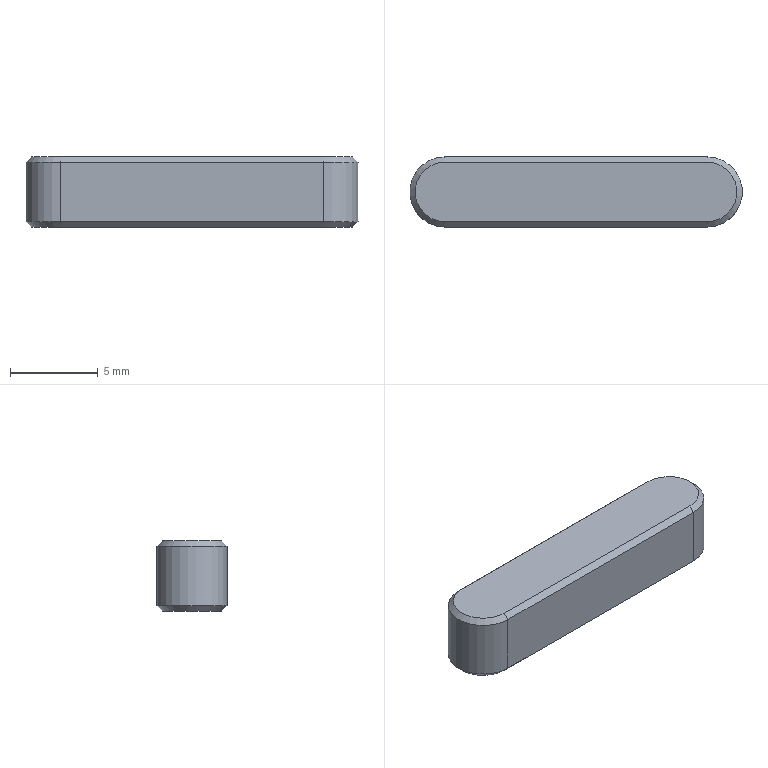Part | NX | 1 solid | 14 faces | box 19 x 4 x 4 mm | volume 286.491 mm3 | plane 8 | cone 4 | cylinder 2 | commonest cylinder face diameters 4 x2
STEP:
#1=CARTESIAN_POINT('',(7.5,2.,3.7));
#2=VERTEX_POINT('',#1);
#3=CARTESIAN_POINT('',(7.5,2.,0.3));
#4=VERTEX_POINT('',#3);
#5=CARTESIAN_POINT('',(7.5,2.,4.));
#6=DIRECTION('',(0.,0.,-1.));
#7=VECTOR('',#6,1000.);
#8=LINE('',#5,#7);
#9=EDGE_CURVE('',#2,#4,#8,.T.);
#10=ORIENTED_EDGE('',*,*,#9,.F.);
#11=CARTESIAN_POINT('',(7.5,-2.,3.7));
#12=VERTEX_POINT('',#11);
#13=CARTESIAN_POINT('',(7.5,0.,3.7));
#14=DIRECTION('',(0.,0.,1.));
#15=DIRECTION('',(1.,0.,0.));
#16=AXIS2_PLACEMENT_3D('',#13,#14,#15);
#17=CIRCLE('',#16,2.);
#18=EDGE_CURVE('',#2,#12,#17,.F.);
#19=ORIENTED_EDGE('',*,*,#18,.T.);
#20=CARTESIAN_POINT('',(7.5,-2.,0.3));
#21=VERTEX_POINT('',#20);
#22=CARTESIAN_POINT('',(7.5,-2.,4.));
#23=DIRECTION('',(0.,0.,-1.));
#24=VECTOR('',#23,1000.);
#25=LINE('',#22,#24);
#26=EDGE_CURVE('',#12,#21,#25,.T.);
#27=ORIENTED_EDGE('',*,*,#26,.T.);
#28=CARTESIAN_POINT('',(7.5,0.,0.3));
#29=DIRECTION('',(0.,0.,1.));
#30=DIRECTION('',(1.,0.,0.));
#31=AXIS2_PLACEMENT_3D('',#28,#29,#30);
#32=CIRCLE('',#31,2.);
#33=EDGE_CURVE('',#21,#4,#32,.T.);
#34=ORIENTED_EDGE('',*,*,#33,.T.);
#35=EDGE_LOOP('',(#10,#19,#27,#34));
#36=FACE_BOUND('',#35,.T.);
#37=CARTESIAN_POINT('',(7.5,0.,4.));
#38=DIRECTION('',(0.,0.,-1.));
#39=DIRECTION('',(-1.,0.,0.));
#40=AXIS2_PLACEMENT_3D('',#37,#38,#39);
#41=CYLINDRICAL_SURFACE('',#40,2.);
#42=ADVANCED_FACE('',(#36),#41,.T.);
#43=CARTESIAN_POINT('',(-7.5,2.,3.7));
#44=VERTEX_POINT('',#43);
#45=CARTESIAN_POINT('',(-7.5,2.,0.3));
#46=VERTEX_POINT('',#45);
#47=CARTESIAN_POINT('',(-7.5,2.,4.));
#48=DIRECTION('',(0.,0.,-1.));
#49=VECTOR('',#48,1000.);
#50=LINE('',#47,#49);
#51=EDGE_CURVE('',#44,#46,#50,.T.);
#52=ORIENTED_EDGE('',*,*,#51,.F.);
#53=CARTESIAN_POINT('',(7.5,2.,3.7));
#54=DIRECTION('',(1.,0.,0.));
#55=VECTOR('',#54,1000.);
#56=LINE('',#53,#55);
#57=EDGE_CURVE('',#44,#2,#56,.T.);
#58=ORIENTED_EDGE('',*,*,#57,.T.);
#59=ORIENTED_EDGE('',*,*,#9,.T.);
#60=CARTESIAN_POINT('',(7.5,2.,0.3));
#61=DIRECTION('',(-1.,0.,0.));
#62=VECTOR('',#61,1000.);
#63=LINE('',#60,#62);
#64=EDGE_CURVE('',#4,#46,#63,.T.);
#65=ORIENTED_EDGE('',*,*,#64,.T.);
#66=EDGE_LOOP('',(#52,#58,#59,#65));
#67=FACE_BOUND('',#66,.T.);
#68=CARTESIAN_POINT('',(7.5,2.,4.));
#69=DIRECTION('',(0.,-1.,0.));
#70=DIRECTION('',(1.,0.,0.));
#71=AXIS2_PLACEMENT_3D('',#68,#69,#70);
#72=PLANE('',#71);
#73=ADVANCED_FACE('',(#67),#72,.F.);
#74=CARTESIAN_POINT('',(-7.5,-2.,3.7));
#75=VERTEX_POINT('',#74);
#76=CARTESIAN_POINT('',(-7.5,-2.,0.3));
#77=VERTEX_POINT('',#76);
#78=CARTESIAN_POINT('',(-7.5,-2.,4.));
#79=DIRECTION('',(0.,0.,-1.));
#80=VECTOR('',#79,1000.);
#81=LINE('',#78,#80);
#82=EDGE_CURVE('',#75,#77,#81,.T.);
#83=ORIENTED_EDGE('',*,*,#82,.F.);
#84=CARTESIAN_POINT('',(-7.5,0.,3.7));
#85=DIRECTION('',(0.,0.,1.));
#86=DIRECTION('',(1.,0.,0.));
#87=AXIS2_PLACEMENT_3D('',#84,#85,#86);
#88=CIRCLE('',#87,2.);
#89=EDGE_CURVE('',#75,#44,#88,.F.);
#90=ORIENTED_EDGE('',*,*,#89,.T.);
#91=ORIENTED_EDGE('',*,*,#51,.T.);
#92=CARTESIAN_POINT('',(-7.5,0.,0.3));
#93=DIRECTION('',(0.,0.,1.));
#94=DIRECTION('',(1.,0.,0.));
#95=AXIS2_PLACEMENT_3D('',#92,#93,#94);
#96=CIRCLE('',#95,2.);
#97=EDGE_CURVE('',#46,#77,#96,.T.);
#98=ORIENTED_EDGE('',*,*,#97,.T.);
#99=EDGE_LOOP('',(#83,#90,#91,#98));
#100=FACE_BOUND('',#99,.T.);
#101=CARTESIAN_POINT('',(-7.5,0.,4.));
#102=DIRECTION('',(0.,0.,-1.));
#103=DIRECTION('',(-1.,0.,0.));
#104=AXIS2_PLACEMENT_3D('',#101,#102,#103);
#105=CYLINDRICAL_SURFACE('',#104,2.);
#106=ADVANCED_FACE('',(#100),#105,.T.);
#107=ORIENTED_EDGE('',*,*,#26,.F.);
#108=CARTESIAN_POINT('',(-7.5,-2.,3.7));
#109=DIRECTION('',(-1.,0.,0.));
#110=VECTOR('',#109,1000.);
#111=LINE('',#108,#110);
#112=EDGE_CURVE('',#12,#75,#111,.T.);
#113=ORIENTED_EDGE('',*,*,#112,.T.);
#114=ORIENTED_EDGE('',*,*,#82,.T.);
#115=CARTESIAN_POINT('',(7.5,-2.,0.3));
#116=DIRECTION('',(1.,0.,0.));
#117=VECTOR('',#116,1000.);
#118=LINE('',#115,#117);
#119=EDGE_CURVE('',#77,#21,#118,.T.);
#120=ORIENTED_EDGE('',*,*,#119,.T.);
#121=EDGE_LOOP('',(#107,#113,#114,#120));
#122=FACE_BOUND('',#121,.T.);
#123=CARTESIAN_POINT('',(7.5,-2.,4.));
#124=DIRECTION('',(0.,1.,0.));
#125=DIRECTION('',(-1.,0.,0.));
#126=AXIS2_PLACEMENT_3D('',#123,#124,#125);
#127=PLANE('',#126);
#128=ADVANCED_FACE('',(#122),#127,.F.);
#129=CARTESIAN_POINT('',(7.5,-1.7,4.));
#130=VERTEX_POINT('',#129);
#131=CARTESIAN_POINT('',(7.5,1.7,4.));
#132=VERTEX_POINT('',#131);
#133=CARTESIAN_POINT('',(7.5,0.,4.));
#134=DIRECTION('',(0.,0.,1.));
#135=DIRECTION('',(1.,0.,0.));
#136=AXIS2_PLACEMENT_3D('',#133,#134,#135);
#137=CIRCLE('',#136,1.7);
#138=EDGE_CURVE('',#130,#132,#137,.T.);
#139=ORIENTED_EDGE('',*,*,#138,.T.);
#140=CARTESIAN_POINT('',(-7.5,1.7,4.));
#141=VERTEX_POINT('',#140);
#142=CARTESIAN_POINT('',(-7.5,1.7,4.));
#143=DIRECTION('',(-1.,0.,0.));
#144=VECTOR('',#143,1000.);
#145=LINE('',#142,#144);
#146=EDGE_CURVE('',#132,#141,#145,.T.);
#147=ORIENTED_EDGE('',*,*,#146,.T.);
#148=CARTESIAN_POINT('',(-7.5,-1.7,4.));
#149=VERTEX_POINT('',#148);
#150=CARTESIAN_POINT('',(-7.5,0.,4.));
#151=DIRECTION('',(0.,0.,1.));
#152=DIRECTION('',(1.,0.,0.));
#153=AXIS2_PLACEMENT_3D('',#150,#151,#152);
#154=CIRCLE('',#153,1.7);
#155=EDGE_CURVE('',#141,#149,#154,.T.);
#156=ORIENTED_EDGE('',*,*,#155,.T.);
#157=CARTESIAN_POINT('',(7.5,-1.7,4.));
#158=DIRECTION('',(1.,0.,0.));
#159=VECTOR('',#158,1000.);
#160=LINE('',#157,#159);
#161=EDGE_CURVE('',#149,#130,#160,.T.);
#162=ORIENTED_EDGE('',*,*,#161,.T.);
#163=EDGE_LOOP('',(#139,#147,#156,#162));
#164=FACE_BOUND('',#163,.T.);
#165=CARTESIAN_POINT('',(7.5,0.,4.));
#166=DIRECTION('',(0.,0.,1.));
#167=DIRECTION('',(1.,0.,0.));
#168=AXIS2_PLACEMENT_3D('',#165,#166,#167);
#169=PLANE('',#168);
#170=ADVANCED_FACE('',(#164),#169,.T.);
#171=CARTESIAN_POINT('',(-7.5,-1.7,0.));
#172=VERTEX_POINT('',#171);
#173=CARTESIAN_POINT('',(-7.5,1.7,0.));
#174=VERTEX_POINT('',#173);
#175=CARTESIAN_POINT('',(-7.5,0.,0.));
#176=DIRECTION('',(0.,0.,1.));
#177=DIRECTION('',(1.,0.,0.));
#178=AXIS2_PLACEMENT_3D('',#175,#176,#177);
#179=CIRCLE('',#178,1.7);
#180=EDGE_CURVE('',#172,#174,#179,.F.);
#181=ORIENTED_EDGE('',*,*,#180,.T.);
#182=CARTESIAN_POINT('',(7.5,1.7,0.));
#183=VERTEX_POINT('',#182);
#184=CARTESIAN_POINT('',(7.5,1.7,0.));
#185=DIRECTION('',(1.,0.,0.));
#186=VECTOR('',#185,1000.);
#187=LINE('',#184,#186);
#188=EDGE_CURVE('',#174,#183,#187,.T.);
#189=ORIENTED_EDGE('',*,*,#188,.T.);
#190=CARTESIAN_POINT('',(7.5,-1.7,0.));
#191=VERTEX_POINT('',#190);
#192=CARTESIAN_POINT('',(7.5,0.,0.));
#193=DIRECTION('',(0.,0.,1.));
#194=DIRECTION('',(1.,0.,0.));
#195=AXIS2_PLACEMENT_3D('',#192,#193,#194);
#196=CIRCLE('',#195,1.7);
#197=EDGE_CURVE('',#183,#191,#196,.F.);
#198=ORIENTED_EDGE('',*,*,#197,.T.);
#199=CARTESIAN_POINT('',(7.5,-1.7,0.));
#200=DIRECTION('',(-1.,0.,0.));
#201=VECTOR('',#200,1000.);
#202=LINE('',#199,#201);
#203=EDGE_CURVE('',#191,#172,#202,.T.);
#204=ORIENTED_EDGE('',*,*,#203,.T.);
#205=EDGE_LOOP('',(#181,#189,#198,#204));
#206=FACE_BOUND('',#205,.T.);
#207=CARTESIAN_POINT('',(7.5,0.,0.));
#208=DIRECTION('',(0.,0.,1.));
#209=DIRECTION('',(1.,0.,0.));
#210=AXIS2_PLACEMENT_3D('',#207,#208,#209);
#211=PLANE('',#210);
#212=ADVANCED_FACE('',(#206),#211,.F.);
#213=CARTESIAN_POINT('',(-7.5,-2.,3.7));
#214=DIRECTION('',(0.,0.7071,0.7071));
#215=VECTOR('',#214,1000.);
#216=LINE('',#213,#215);
#217=EDGE_CURVE('',#75,#149,#216,.T.);
#218=ORIENTED_EDGE('',*,*,#217,.F.);
#219=ORIENTED_EDGE('',*,*,#112,.F.);
#220=CARTESIAN_POINT('',(7.5,-1.7,4.));
#221=DIRECTION('',(0.,-0.7071,-0.7071));
#222=VECTOR('',#221,1000.);
#223=LINE('',#220,#222);
#224=EDGE_CURVE('',#130,#12,#223,.T.);
#225=ORIENTED_EDGE('',*,*,#224,.F.);
#226=ORIENTED_EDGE('',*,*,#161,.F.);
#227=EDGE_LOOP('',(#218,#219,#225,#226));
#228=FACE_BOUND('',#227,.T.);
#229=CARTESIAN_POINT('',(7.5,-1.7,4.));
#230=DIRECTION('',(0.,-0.7071,0.7071));
#231=DIRECTION('',(-1.,0.,0.));
#232=AXIS2_PLACEMENT_3D('',#229,#230,#231);
#233=PLANE('',#232);
#234=ADVANCED_FACE('',(#228),#233,.T.);
#235=ORIENTED_EDGE('',*,*,#224,.T.);
#236=ORIENTED_EDGE('',*,*,#18,.F.);
#237=CARTESIAN_POINT('',(7.5,1.7,4.));
#238=DIRECTION('',(0.,0.7071,-0.7071));
#239=VECTOR('',#238,1000.);
#240=LINE('',#237,#239);
#241=EDGE_CURVE('',#132,#2,#240,.T.);
#242=ORIENTED_EDGE('',*,*,#241,.F.);
#243=ORIENTED_EDGE('',*,*,#138,.F.);
#244=EDGE_LOOP('',(#235,#236,#242,#243));
#245=FACE_BOUND('',#244,.T.);
#246=CARTESIAN_POINT('',(7.5,0.,4.));
#247=DIRECTION('',(0.,0.,-1.));
#248=DIRECTION('',(-1.,0.,0.));
#249=AXIS2_PLACEMENT_3D('',#246,#247,#248);
#250=CONICAL_SURFACE('',#249,1.7,0.7854);
#251=ADVANCED_FACE('',(#245),#250,.T.);
#252=ORIENTED_EDGE('',*,*,#217,.T.);
#253=ORIENTED_EDGE('',*,*,#155,.F.);
#254=CARTESIAN_POINT('',(-7.5,2.,3.7));
#255=DIRECTION('',(0.,-0.7071,0.7071));
#256=VECTOR('',#255,1000.);
#257=LINE('',#254,#256);
#258=EDGE_CURVE('',#44,#141,#257,.T.);
#259=ORIENTED_EDGE('',*,*,#258,.F.);
#260=ORIENTED_EDGE('',*,*,#89,.F.);
#261=EDGE_LOOP('',(#252,#253,#259,#260));
#262=FACE_BOUND('',#261,.T.);
#263=CARTESIAN_POINT('',(-7.5,0.,4.));
#264=DIRECTION('',(0.,0.,-1.));
#265=DIRECTION('',(-1.,0.,0.));
#266=AXIS2_PLACEMENT_3D('',#263,#264,#265);
#267=CONICAL_SURFACE('',#266,1.7,0.7854);
#268=ADVANCED_FACE('',(#262),#267,.T.);
#269=ORIENTED_EDGE('',*,*,#241,.T.);
#270=ORIENTED_EDGE('',*,*,#57,.F.);
#271=ORIENTED_EDGE('',*,*,#258,.T.);
#272=ORIENTED_EDGE('',*,*,#146,.F.);
#273=EDGE_LOOP('',(#269,#270,#271,#272));
#274=FACE_BOUND('',#273,.T.);
#275=CARTESIAN_POINT('',(7.5,1.7,4.));
#276=DIRECTION('',(0.,0.7071,0.7071));
#277=DIRECTION('',(1.,0.,0.));
#278=AXIS2_PLACEMENT_3D('',#275,#276,#277);
#279=PLANE('',#278);
#280=ADVANCED_FACE('',(#274),#279,.T.);
#281=CARTESIAN_POINT('',(-7.5,-1.7,0.));
#282=DIRECTION('',(0.,-0.7071,0.7071));
#283=VECTOR('',#282,1000.);
#284=LINE('',#281,#283);
#285=EDGE_CURVE('',#172,#77,#284,.T.);
#286=ORIENTED_EDGE('',*,*,#285,.F.);
#287=ORIENTED_EDGE('',*,*,#203,.F.);
#288=CARTESIAN_POINT('',(7.5,-2.,0.3));
#289=DIRECTION('',(0.,0.7071,-0.7071));
#290=VECTOR('',#289,1000.);
#291=LINE('',#288,#290);
#292=EDGE_CURVE('',#21,#191,#291,.T.);
#293=ORIENTED_EDGE('',*,*,#292,.F.);
#294=ORIENTED_EDGE('',*,*,#119,.F.);
#295=EDGE_LOOP('',(#286,#287,#293,#294));
#296=FACE_BOUND('',#295,.T.);
#297=CARTESIAN_POINT('',(7.5,-2.,0.3));
#298=DIRECTION('',(0.,0.7071,0.7071));
#299=DIRECTION('',(1.,0.,0.));
#300=AXIS2_PLACEMENT_3D('',#297,#298,#299);
#301=PLANE('',#300);
#302=ADVANCED_FACE('',(#296),#301,.F.);
#303=ORIENTED_EDGE('',*,*,#292,.T.);
#304=ORIENTED_EDGE('',*,*,#197,.F.);
#305=CARTESIAN_POINT('',(7.5,2.,0.3));
#306=DIRECTION('',(0.,-0.7071,-0.7071));
#307=VECTOR('',#306,1000.);
#308=LINE('',#305,#307);
#309=EDGE_CURVE('',#4,#183,#308,.T.);
#310=ORIENTED_EDGE('',*,*,#309,.F.);
#311=ORIENTED_EDGE('',*,*,#33,.F.);
#312=EDGE_LOOP('',(#303,#304,#310,#311));
#313=FACE_BOUND('',#312,.T.);
#314=CARTESIAN_POINT('',(7.5,0.,0.3));
#315=DIRECTION('',(0.,0.,1.));
#316=DIRECTION('',(1.,0.,0.));
#317=AXIS2_PLACEMENT_3D('',#314,#315,#316);
#318=CONICAL_SURFACE('',#317,2.,0.7854);
#319=ADVANCED_FACE('',(#313),#318,.T.);
#320=ORIENTED_EDGE('',*,*,#285,.T.);
#321=ORIENTED_EDGE('',*,*,#97,.F.);
#322=CARTESIAN_POINT('',(-7.5,1.7,0.));
#323=DIRECTION('',(0.,0.7071,0.7071));
#324=VECTOR('',#323,1000.);
#325=LINE('',#322,#324);
#326=EDGE_CURVE('',#174,#46,#325,.T.);
#327=ORIENTED_EDGE('',*,*,#326,.F.);
#328=ORIENTED_EDGE('',*,*,#180,.F.);
#329=EDGE_LOOP('',(#320,#321,#327,#328));
#330=FACE_BOUND('',#329,.T.);
#331=CARTESIAN_POINT('',(-7.5,0.,0.3));
#332=DIRECTION('',(0.,0.,1.));
#333=DIRECTION('',(1.,0.,0.));
#334=AXIS2_PLACEMENT_3D('',#331,#332,#333);
#335=CONICAL_SURFACE('',#334,2.,0.7854);
#336=ADVANCED_FACE('',(#330),#335,.T.);
#337=ORIENTED_EDGE('',*,*,#309,.T.);
#338=ORIENTED_EDGE('',*,*,#188,.F.);
#339=ORIENTED_EDGE('',*,*,#326,.T.);
#340=ORIENTED_EDGE('',*,*,#64,.F.);
#341=EDGE_LOOP('',(#337,#338,#339,#340));
#342=FACE_BOUND('',#341,.T.);
#343=CARTESIAN_POINT('',(7.5,2.,0.3));
#344=DIRECTION('',(0.,-0.7071,0.7071));
#345=DIRECTION('',(-1.,0.,0.));
#346=AXIS2_PLACEMENT_3D('',#343,#344,#345);
#347=PLANE('',#346);
#348=ADVANCED_FACE('',(#342),#347,.F.);
#349=CLOSED_SHELL('',(#42,#73,#106,#128,#170,#212,#234,#251,#268,#280,#302,#319,#336,#348));
#350=MANIFOLD_SOLID_BREP('',#349);
#351=(LENGTH_UNIT()NAMED_UNIT(*)SI_UNIT(.MILLI.,.METRE.));
#352=UNCERTAINTY_MEASURE_WITH_UNIT(LENGTH_MEASURE(0.00001),#351,'','');
#353=(NAMED_UNIT(*)PLANE_ANGLE_UNIT()SI_UNIT($,.RADIAN.));
#354=(NAMED_UNIT(*)SI_UNIT($,.STERADIAN.)SOLID_ANGLE_UNIT());
#355=(GEOMETRIC_REPRESENTATION_CONTEXT(3)GLOBAL_UNCERTAINTY_ASSIGNED_CONTEXT((#352))GLOBAL_UNIT_ASSIGNED_CONTEXT((#351,#353,#354))REPRESENTATION_CONTEXT('',''));
#356=ADVANCED_BREP_SHAPE_REPRESENTATION('',(#350),#355);